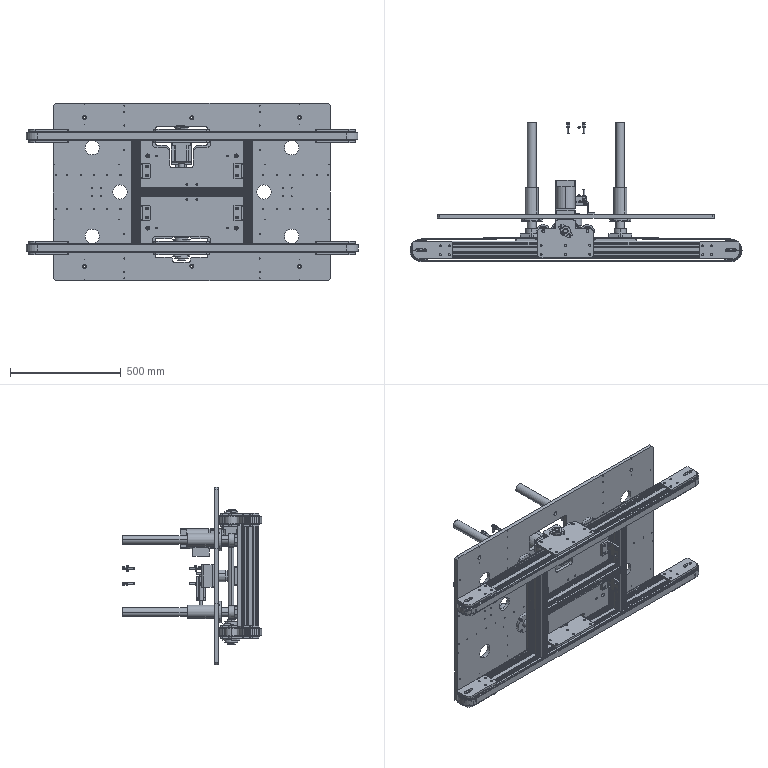Part | SolidWorks | 95 solids | 7645 faces | volume 34812843 mm3 | cylinder 2901 | plane 2700 | torus 902 | sphere 512 | cone 448 | spline 182 | commonest cylinder face diameters 1.2 x452 1.6 x452 5 x162 9 x142 10 x130 93.64 x124